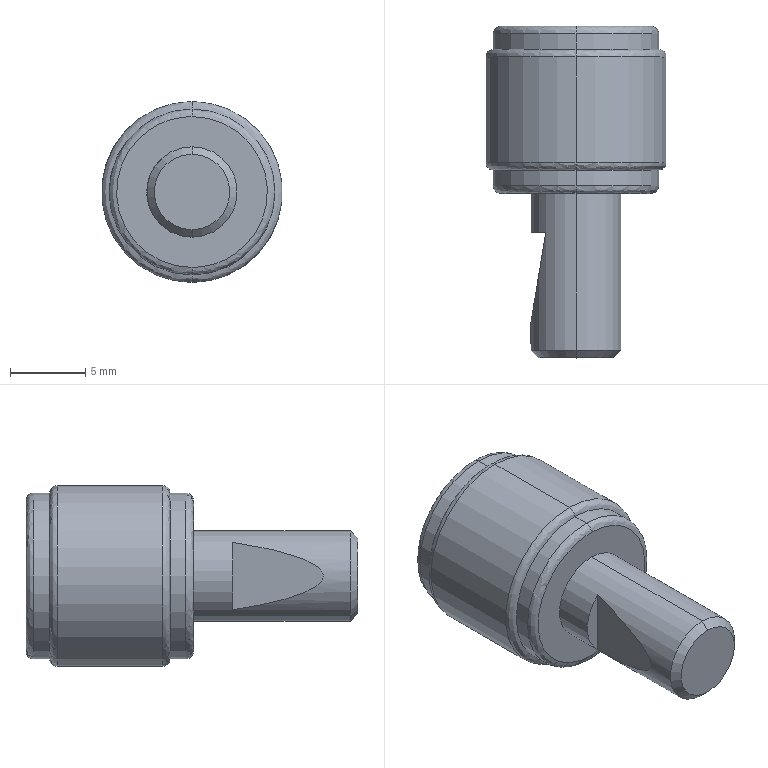Part | SolidWorks | features BaseBody 1 | 1 solid | 30 faces | box 12 x 22 x 12 mm | volume 1467 mm3 | plane 12 | spline 8 | cylinder 8 | cone 2 | commonest cylinder face diameters 11 x4 6 x2 12 x2
STEP:
#1=CARTESIAN_POINT('',(0.,20.45,5.5));
#2=VERTEX_POINT('',#1);
#3=CARTESIAN_POINT('',(0.,20.45,-5.5));
#4=VERTEX_POINT('',#3);
#5=CARTESIAN_POINT('',(0.,20.45,0.));
#6=DIRECTION('',(0.,-1.,0.));
#7=DIRECTION('',(0.,0.,1.));
#8=AXIS2_PLACEMENT_3D('',#5,#6,#7);
#9=CIRCLE('',#8,5.5);
#10=EDGE_CURVE('',#2,#4,#9,.T.);
#11=ORIENTED_EDGE('',*,*,#10,.T.);
#12=CARTESIAN_POINT('',(0.,19.95,-6.));
#13=VERTEX_POINT('',#12);
#14=CARTESIAN_POINT('',(0.,19.95,-5.5));
#15=DIRECTION('',(-1.,0.,0.));
#16=DIRECTION('',(0.,0.,-1.));
#17=AXIS2_PLACEMENT_3D('',#14,#15,#16);
#18=CIRCLE('',#17,0.5);
#19=EDGE_CURVE('',#4,#13,#18,.T.);
#20=ORIENTED_EDGE('',*,*,#19,.T.);
#21=CARTESIAN_POINT('',(0.,19.95,6.));
#22=VERTEX_POINT('',#21);
#23=CARTESIAN_POINT('',(0.,19.95,0.));
#24=DIRECTION('',(0.,-1.,0.));
#25=DIRECTION('',(0.,0.,1.));
#26=AXIS2_PLACEMENT_3D('',#23,#24,#25);
#27=CIRCLE('',#26,6.);
#28=EDGE_CURVE('',#22,#13,#27,.T.);
#29=ORIENTED_EDGE('',*,*,#28,.F.);
#30=CARTESIAN_POINT('',(0.,19.95,5.5));
#31=DIRECTION('',(1.,0.,0.));
#32=DIRECTION('',(0.,0.,1.));
#33=AXIS2_PLACEMENT_3D('',#30,#31,#32);
#34=CIRCLE('',#33,0.5);
#35=EDGE_CURVE('',#2,#22,#34,.T.);
#36=ORIENTED_EDGE('',*,*,#35,.F.);
#37=EDGE_LOOP('',(#11,#20,#29,#36));
#38=FACE_OUTER_BOUND('',#37,.T.);
#39=CARTESIAN_POINT('',(0.,20.45,-5.5));
#40=CARTESIAN_POINT('',(-11.,20.45,-5.5));
#41=CARTESIAN_POINT('',(-11.,20.45,5.5));
#42=CARTESIAN_POINT('',(0.,20.45,5.5));
#43=CARTESIAN_POINT('',(0.,20.45,-5.793));
#44=CARTESIAN_POINT('',(-11.586,20.45,-5.793));
#45=CARTESIAN_POINT('',(-11.586,20.45,5.793));
#46=CARTESIAN_POINT('',(0.,20.45,5.793));
#47=CARTESIAN_POINT('',(0.,20.243,-6.));
#48=CARTESIAN_POINT('',(-12.,20.243,-6.));
#49=CARTESIAN_POINT('',(-12.,20.243,6.));
#50=CARTESIAN_POINT('',(0.,20.243,6.));
#51=CARTESIAN_POINT('',(0.,19.95,-6.));
#52=CARTESIAN_POINT('',(-12.,19.95,-6.));
#53=CARTESIAN_POINT('',(-12.,19.95,6.));
#54=CARTESIAN_POINT('',(0.,19.95,6.));
#55=(BOUNDED_SURFACE()B_SPLINE_SURFACE(3,3,((#39,#40,#41,#42),(#43,#44,#45,#46),(#47,#48,#49,#50),(#51,#52,#53,#54)),.UNSPECIFIED.,.F.,.F.,.F.)B_SPLINE_SURFACE_WITH_KNOTS((4,4),(4,4),(0.,1.),(0.,1.),.UNSPECIFIED.)GEOMETRIC_REPRESENTATION_ITEM()RATIONAL_B_SPLINE_SURFACE(((1.,0.3333,0.3333,1.),(0.8047,0.2682,0.2682,0.8047),(0.8047,0.2682,0.2682,0.8047),(1.,0.3333,0.3333,1.)))REPRESENTATION_ITEM('')SURFACE());
#56=ADVANCED_FACE('',(#38),#55,.T.);
#57=CARTESIAN_POINT('',(0.,12.45,-5.5));
#58=VERTEX_POINT('',#57);
#59=CARTESIAN_POINT('',(0.,12.45,5.5));
#60=VERTEX_POINT('',#59);
#61=CARTESIAN_POINT('',(0.,12.45,0.));
#62=DIRECTION('',(0.,1.,0.));
#63=DIRECTION('',(0.,0.,-1.));
#64=AXIS2_PLACEMENT_3D('',#61,#62,#63);
#65=CIRCLE('',#64,5.5);
#66=EDGE_CURVE('',#58,#60,#65,.T.);
#67=ORIENTED_EDGE('',*,*,#66,.T.);
#68=CARTESIAN_POINT('',(0.,12.95,6.));
#69=VERTEX_POINT('',#68);
#70=CARTESIAN_POINT('',(0.,12.95,5.5));
#71=DIRECTION('',(-1.,0.,0.));
#72=DIRECTION('',(0.,0.,1.));
#73=AXIS2_PLACEMENT_3D('',#70,#71,#72);
#74=CIRCLE('',#73,0.5);
#75=EDGE_CURVE('',#60,#69,#74,.T.);
#76=ORIENTED_EDGE('',*,*,#75,.T.);
#77=CARTESIAN_POINT('',(0.,12.95,-6.));
#78=VERTEX_POINT('',#77);
#79=CARTESIAN_POINT('',(0.,12.95,0.));
#80=DIRECTION('',(0.,1.,0.));
#81=DIRECTION('',(0.,0.,1.));
#82=AXIS2_PLACEMENT_3D('',#79,#80,#81);
#83=CIRCLE('',#82,6.);
#84=EDGE_CURVE('',#78,#69,#83,.T.);
#85=ORIENTED_EDGE('',*,*,#84,.F.);
#86=CARTESIAN_POINT('',(0.,12.95,-5.5));
#87=DIRECTION('',(1.,0.,0.));
#88=DIRECTION('',(0.,0.,-1.));
#89=AXIS2_PLACEMENT_3D('',#86,#87,#88);
#90=CIRCLE('',#89,0.5);
#91=EDGE_CURVE('',#58,#78,#90,.T.);
#92=ORIENTED_EDGE('',*,*,#91,.F.);
#93=EDGE_LOOP('',(#67,#76,#85,#92));
#94=FACE_OUTER_BOUND('',#93,.T.);
#95=CARTESIAN_POINT('',(0.,12.45,5.5));
#96=CARTESIAN_POINT('',(-11.,12.45,5.5));
#97=CARTESIAN_POINT('',(-11.,12.45,-5.5));
#98=CARTESIAN_POINT('',(0.,12.45,-5.5));
#99=CARTESIAN_POINT('',(0.,12.45,5.793));
#100=CARTESIAN_POINT('',(-11.586,12.45,5.793));
#101=CARTESIAN_POINT('',(-11.586,12.45,-5.793));
#102=CARTESIAN_POINT('',(0.,12.45,-5.793));
#103=CARTESIAN_POINT('',(0.,12.657,6.));
#104=CARTESIAN_POINT('',(-12.,12.657,6.));
#105=CARTESIAN_POINT('',(-12.,12.657,-6.));
#106=CARTESIAN_POINT('',(0.,12.657,-6.));
#107=CARTESIAN_POINT('',(0.,12.95,6.));
#108=CARTESIAN_POINT('',(-12.,12.95,6.));
#109=CARTESIAN_POINT('',(-12.,12.95,-6.));
#110=CARTESIAN_POINT('',(0.,12.95,-6.));
#111=(BOUNDED_SURFACE()B_SPLINE_SURFACE(3,3,((#95,#96,#97,#98),(#99,#100,#101,#102),(#103,#104,#105,#106),(#107,#108,#109,#110)),.UNSPECIFIED.,.F.,.F.,.F.)B_SPLINE_SURFACE_WITH_KNOTS((4,4),(4,4),(0.,1.),(0.,1.),.UNSPECIFIED.)GEOMETRIC_REPRESENTATION_ITEM()RATIONAL_B_SPLINE_SURFACE(((1.,0.3333,0.3333,1.),(0.8047,0.2682,0.2682,0.8047),(0.8047,0.2682,0.2682,0.8047),(1.,0.3333,0.3333,1.)))REPRESENTATION_ITEM('')SURFACE());
#112=ADVANCED_FACE('',(#94),#111,.T.);
#113=CARTESIAN_POINT('',(0.,22.,5.));
#114=VERTEX_POINT('',#113);
#115=CARTESIAN_POINT('',(0.,22.,-5.));
#116=VERTEX_POINT('',#115);
#117=CARTESIAN_POINT('',(0.,22.,5.));
#118=CARTESIAN_POINT('',(-10.,22.,5.));
#119=CARTESIAN_POINT('',(-10.,22.,-5.));
#120=CARTESIAN_POINT('',(0.,22.,-5.));
#121=(BOUNDED_CURVE()B_SPLINE_CURVE(3,(#117,#118,#119,#120),.UNSPECIFIED.,.F.,.F.)B_SPLINE_CURVE_WITH_KNOTS((4,4),(0.,1.),.UNSPECIFIED.)CURVE()GEOMETRIC_REPRESENTATION_ITEM()RATIONAL_B_SPLINE_CURVE((1.,0.3333,0.3333,1.))REPRESENTATION_ITEM(''));
#122=EDGE_CURVE('',#114,#116,#121,.T.);
#123=ORIENTED_EDGE('',*,*,#122,.T.);
#124=CARTESIAN_POINT('',(0.,21.5,-5.5));
#125=VERTEX_POINT('',#124);
#126=CARTESIAN_POINT('',(0.,21.5,-5.));
#127=DIRECTION('',(-1.,0.,0.));
#128=DIRECTION('',(0.,0.,-1.));
#129=AXIS2_PLACEMENT_3D('',#126,#127,#128);
#130=CIRCLE('',#129,0.5);
#131=EDGE_CURVE('',#116,#125,#130,.T.);
#132=ORIENTED_EDGE('',*,*,#131,.T.);
#133=CARTESIAN_POINT('',(0.,21.5,5.5));
#134=VERTEX_POINT('',#133);
#135=CARTESIAN_POINT('',(0.,21.5,0.));
#136=DIRECTION('',(0.,-1.,0.));
#137=DIRECTION('',(0.,0.,1.));
#138=AXIS2_PLACEMENT_3D('',#135,#136,#137);
#139=CIRCLE('',#138,5.5);
#140=EDGE_CURVE('',#134,#125,#139,.T.);
#141=ORIENTED_EDGE('',*,*,#140,.F.);
#142=CARTESIAN_POINT('',(0.,21.5,5.));
#143=DIRECTION('',(1.,0.,0.));
#144=DIRECTION('',(0.,0.,1.));
#145=AXIS2_PLACEMENT_3D('',#142,#143,#144);
#146=CIRCLE('',#145,0.5);
#147=EDGE_CURVE('',#114,#134,#146,.T.);
#148=ORIENTED_EDGE('',*,*,#147,.F.);
#149=EDGE_LOOP('',(#123,#132,#141,#148));
#150=FACE_OUTER_BOUND('',#149,.T.);
#151=CARTESIAN_POINT('',(0.,22.,-5.));
#152=CARTESIAN_POINT('',(-10.,22.,-5.));
#153=CARTESIAN_POINT('',(-10.,22.,5.));
#154=CARTESIAN_POINT('',(0.,22.,5.));
#155=CARTESIAN_POINT('',(0.,22.,-5.293));
#156=CARTESIAN_POINT('',(-10.586,22.,-5.293));
#157=CARTESIAN_POINT('',(-10.586,22.,5.293));
#158=CARTESIAN_POINT('',(0.,22.,5.293));
#159=CARTESIAN_POINT('',(0.,21.793,-5.5));
#160=CARTESIAN_POINT('',(-11.,21.793,-5.5));
#161=CARTESIAN_POINT('',(-11.,21.793,5.5));
#162=CARTESIAN_POINT('',(0.,21.793,5.5));
#163=CARTESIAN_POINT('',(0.,21.5,-5.5));
#164=CARTESIAN_POINT('',(-11.,21.5,-5.5));
#165=CARTESIAN_POINT('',(-11.,21.5,5.5));
#166=CARTESIAN_POINT('',(0.,21.5,5.5));
#167=(BOUNDED_SURFACE()B_SPLINE_SURFACE(3,3,((#151,#152,#153,#154),(#155,#156,#157,#158),(#159,#160,#161,#162),(#163,#164,#165,#166)),.UNSPECIFIED.,.F.,.F.,.F.)B_SPLINE_SURFACE_WITH_KNOTS((4,4),(4,4),(0.,1.),(0.,1.),.UNSPECIFIED.)GEOMETRIC_REPRESENTATION_ITEM()RATIONAL_B_SPLINE_SURFACE(((1.,0.3333,0.3333,1.),(0.8047,0.2682,0.2682,0.8047),(0.8047,0.2682,0.2682,0.8047),(1.,0.3333,0.3333,1.)))REPRESENTATION_ITEM('')SURFACE());
#168=ADVANCED_FACE('',(#150),#167,.T.);
#169=CARTESIAN_POINT('',(0.,10.9,-5.));
#170=VERTEX_POINT('',#169);
#171=CARTESIAN_POINT('',(0.,10.9,5.));
#172=VERTEX_POINT('',#171);
#173=CARTESIAN_POINT('',(0.,10.9,-5.));
#174=CARTESIAN_POINT('',(-10.,10.9,-5.));
#175=CARTESIAN_POINT('',(-10.,10.9,5.));
#176=CARTESIAN_POINT('',(0.,10.9,5.));
#177=(BOUNDED_CURVE()B_SPLINE_CURVE(3,(#173,#174,#175,#176),.UNSPECIFIED.,.F.,.F.)B_SPLINE_CURVE_WITH_KNOTS((4,4),(0.,1.),.UNSPECIFIED.)CURVE()GEOMETRIC_REPRESENTATION_ITEM()RATIONAL_B_SPLINE_CURVE((1.,0.3333,0.3333,1.))REPRESENTATION_ITEM(''));
#178=EDGE_CURVE('',#170,#172,#177,.T.);
#179=ORIENTED_EDGE('',*,*,#178,.T.);
#180=CARTESIAN_POINT('',(0.,11.4,5.5));
#181=VERTEX_POINT('',#180);
#182=CARTESIAN_POINT('',(0.,11.4,5.));
#183=DIRECTION('',(-1.,0.,0.));
#184=DIRECTION('',(0.,0.,1.));
#185=AXIS2_PLACEMENT_3D('',#182,#183,#184);
#186=CIRCLE('',#185,0.5);
#187=EDGE_CURVE('',#172,#181,#186,.T.);
#188=ORIENTED_EDGE('',*,*,#187,.T.);
#189=CARTESIAN_POINT('',(0.,11.4,-5.5));
#190=VERTEX_POINT('',#189);
#191=CARTESIAN_POINT('',(0.,11.4,0.));
#192=DIRECTION('',(0.,1.,0.));
#193=DIRECTION('',(0.,0.,1.));
#194=AXIS2_PLACEMENT_3D('',#191,#192,#193);
#195=CIRCLE('',#194,5.5);
#196=EDGE_CURVE('',#190,#181,#195,.T.);
#197=ORIENTED_EDGE('',*,*,#196,.F.);
#198=CARTESIAN_POINT('',(0.,11.4,-5.));
#199=DIRECTION('',(1.,0.,0.));
#200=DIRECTION('',(0.,0.,-1.));
#201=AXIS2_PLACEMENT_3D('',#198,#199,#200);
#202=CIRCLE('',#201,0.5);
#203=EDGE_CURVE('',#170,#190,#202,.T.);
#204=ORIENTED_EDGE('',*,*,#203,.F.);
#205=EDGE_LOOP('',(#179,#188,#197,#204));
#206=FACE_OUTER_BOUND('',#205,.T.);
#207=CARTESIAN_POINT('',(0.,10.9,5.));
#208=CARTESIAN_POINT('',(-10.,10.9,5.));
#209=CARTESIAN_POINT('',(-10.,10.9,-5.));
#210=CARTESIAN_POINT('',(0.,10.9,-5.));
#211=CARTESIAN_POINT('',(0.,10.9,5.293));
#212=CARTESIAN_POINT('',(-10.586,10.9,5.293));
#213=CARTESIAN_POINT('',(-10.586,10.9,-5.293));
#214=CARTESIAN_POINT('',(0.,10.9,-5.293));
#215=CARTESIAN_POINT('',(0.,11.107,5.5));
#216=CARTESIAN_POINT('',(-11.,11.107,5.5));
#217=CARTESIAN_POINT('',(-11.,11.107,-5.5));
#218=CARTESIAN_POINT('',(0.,11.107,-5.5));
#219=CARTESIAN_POINT('',(0.,11.4,5.5));
#220=CARTESIAN_POINT('',(-11.,11.4,5.5));
#221=CARTESIAN_POINT('',(-11.,11.4,-5.5));
#222=CARTESIAN_POINT('',(0.,11.4,-5.5));
#223=(BOUNDED_SURFACE()B_SPLINE_SURFACE(3,3,((#207,#208,#209,#210),(#211,#212,#213,#214),(#215,#216,#217,#218),(#219,#220,#221,#222)),.UNSPECIFIED.,.F.,.F.,.F.)B_SPLINE_SURFACE_WITH_KNOTS((4,4),(4,4),(0.,1.),(0.,1.),.UNSPECIFIED.)GEOMETRIC_REPRESENTATION_ITEM()RATIONAL_B_SPLINE_SURFACE(((1.,0.3333,0.3333,1.),(0.8047,0.2682,0.2682,0.8047),(0.8047,0.2682,0.2682,0.8047),(1.,0.3333,0.3333,1.)))REPRESENTATION_ITEM('')SURFACE());
#224=ADVANCED_FACE('',(#206),#223,.T.);
#225=CARTESIAN_POINT('',(0.,12.95,0.));
#226=DIRECTION('',(0.,1.,0.));
#227=DIRECTION('',(0.,0.,1.));
#228=AXIS2_PLACEMENT_3D('',#225,#226,#227);
#229=CIRCLE('',#228,6.);
#230=EDGE_CURVE('',#69,#78,#229,.T.);
#231=ORIENTED_EDGE('',*,*,#230,.T.);
#232=CARTESIAN_POINT('',(0.,0.,-6.));
#233=DIRECTION('',(0.,1.,0.));
#234=VECTOR('',#233,1000.);
#235=LINE('',#232,#234);
#236=EDGE_CURVE('',#78,#13,#235,.T.);
#237=ORIENTED_EDGE('',*,*,#236,.T.);
#238=CARTESIAN_POINT('',(0.,19.95,0.));
#239=DIRECTION('',(0.,-1.,0.));
#240=DIRECTION('',(0.,0.,1.));
#241=AXIS2_PLACEMENT_3D('',#238,#239,#240);
#242=CIRCLE('',#241,6.);
#243=EDGE_CURVE('',#13,#22,#242,.T.);
#244=ORIENTED_EDGE('',*,*,#243,.T.);
#245=CARTESIAN_POINT('',(0.,0.,6.));
#246=DIRECTION('',(0.,1.,0.));
#247=VECTOR('',#246,1000.);
#248=LINE('',#245,#247);
#249=EDGE_CURVE('',#69,#22,#248,.T.);
#250=ORIENTED_EDGE('',*,*,#249,.F.);
#251=EDGE_LOOP('',(#231,#237,#244,#250));
#252=FACE_OUTER_BOUND('',#251,.T.);
#253=CARTESIAN_POINT('',(0.,0.,0.));
#254=DIRECTION('',(0.,1.,0.));
#255=DIRECTION('',(0.,0.,1.));
#256=AXIS2_PLACEMENT_3D('',#253,#254,#255);
#257=CYLINDRICAL_SURFACE('',#256,6.);
#258=ADVANCED_FACE('',(#252),#257,.T.);
#259=CARTESIAN_POINT('',(0.,20.45,0.));
#260=DIRECTION('',(0.,-1.,0.));
#261=DIRECTION('',(0.,0.,1.));
#262=AXIS2_PLACEMENT_3D('',#259,#260,#261);
#263=CIRCLE('',#262,5.5);
#264=EDGE_CURVE('',#4,#2,#263,.T.);
#265=ORIENTED_EDGE('',*,*,#264,.F.);
#266=CARTESIAN_POINT('',(0.,0.,-5.5));
#267=DIRECTION('',(0.,1.,0.));
#268=VECTOR('',#267,1000.);
#269=LINE('',#266,#268);
#270=EDGE_CURVE('',#4,#125,#269,.T.);
#271=ORIENTED_EDGE('',*,*,#270,.T.);
#272=CARTESIAN_POINT('',(0.,21.5,0.));
#273=DIRECTION('',(0.,-1.,0.));
#274=DIRECTION('',(0.,0.,1.));
#275=AXIS2_PLACEMENT_3D('',#272,#273,#274);
#276=CIRCLE('',#275,5.5);
#277=EDGE_CURVE('',#125,#134,#276,.T.);
#278=ORIENTED_EDGE('',*,*,#277,.T.);
#279=CARTESIAN_POINT('',(0.,0.,5.5));
#280=DIRECTION('',(0.,1.,0.));
#281=VECTOR('',#280,1000.);
#282=LINE('',#279,#281);
#283=EDGE_CURVE('',#2,#134,#282,.T.);
#284=ORIENTED_EDGE('',*,*,#283,.F.);
#285=EDGE_LOOP('',(#265,#271,#278,#284));
#286=FACE_OUTER_BOUND('',#285,.T.);
#287=CARTESIAN_POINT('',(0.,0.,0.));
#288=DIRECTION('',(0.,1.,0.));
#289=DIRECTION('',(0.,0.,1.));
#290=AXIS2_PLACEMENT_3D('',#287,#288,#289);
#291=CYLINDRICAL_SURFACE('',#290,5.5);
#292=ADVANCED_FACE('',(#286),#291,.T.);
#293=CARTESIAN_POINT('',(0.,11.4,0.));
#294=DIRECTION('',(0.,1.,0.));
#295=DIRECTION('',(0.,0.,1.));
#296=AXIS2_PLACEMENT_3D('',#293,#294,#295);
#297=CIRCLE('',#296,5.5);
#298=EDGE_CURVE('',#181,#190,#297,.T.);
#299=ORIENTED_EDGE('',*,*,#298,.T.);
#300=CARTESIAN_POINT('',(0.,0.,-5.5));
#301=DIRECTION('',(0.,1.,0.));
#302=VECTOR('',#301,1000.);
#303=LINE('',#300,#302);
#304=EDGE_CURVE('',#190,#58,#303,.T.);
#305=ORIENTED_EDGE('',*,*,#304,.T.);
#306=CARTESIAN_POINT('',(0.,12.45,0.));
#307=DIRECTION('',(0.,1.,0.));
#308=DIRECTION('',(0.,0.,-1.));
#309=AXIS2_PLACEMENT_3D('',#306,#307,#308);
#310=CIRCLE('',#309,5.5);
#311=EDGE_CURVE('',#60,#58,#310,.T.);
#312=ORIENTED_EDGE('',*,*,#311,.F.);
#313=CARTESIAN_POINT('',(0.,0.,5.5));
#314=DIRECTION('',(0.,1.,0.));
#315=VECTOR('',#314,1000.);
#316=LINE('',#313,#315);
#317=EDGE_CURVE('',#181,#60,#316,.T.);
#318=ORIENTED_EDGE('',*,*,#317,.F.);
#319=EDGE_LOOP('',(#299,#305,#312,#318));
#320=FACE_OUTER_BOUND('',#319,.T.);
#321=CARTESIAN_POINT('',(0.,0.,0.));
#322=DIRECTION('',(0.,1.,0.));
#323=DIRECTION('',(0.,0.,1.));
#324=AXIS2_PLACEMENT_3D('',#321,#322,#323);
#325=CYLINDRICAL_SURFACE('',#324,5.5);
#326=ADVANCED_FACE('',(#320),#325,.T.);
#327=CARTESIAN_POINT('',(0.,0.5,3.));
#328=VERTEX_POINT('',#327);
#329=CARTESIAN_POINT('',(0.,0.5,-3.));
#330=VERTEX_POINT('',#329);
#331=CARTESIAN_POINT('',(0.,0.5,0.));
#332=DIRECTION('',(0.,1.,0.));
#333=DIRECTION('',(0.,0.,1.));
#334=AXIS2_PLACEMENT_3D('',#331,#332,#333);
#335=CIRCLE('',#334,3.);
#336=EDGE_CURVE('',#328,#330,#335,.T.);
#337=ORIENTED_EDGE('',*,*,#336,.T.);
#338=CARTESIAN_POINT('',(0.,10.9,-3.));
#339=VERTEX_POINT('',#338);
#340=CARTESIAN_POINT('',(0.,0.,-3.));
#341=DIRECTION('',(0.,1.,0.));
#342=VECTOR('',#341,1000.);
#343=LINE('',#340,#342);
#344=EDGE_CURVE('',#330,#339,#343,.T.);
#345=ORIENTED_EDGE('',*,*,#344,.T.);
#346=CARTESIAN_POINT('',(0.,10.9,3.));
#347=VERTEX_POINT('',#346);
#348=CARTESIAN_POINT('',(0.,10.9,0.));
#349=DIRECTION('',(0.,1.,0.));
#350=DIRECTION('',(0.,0.,1.));
#351=AXIS2_PLACEMENT_3D('',#348,#349,#350);
#352=CIRCLE('',#351,3.);
#353=EDGE_CURVE('',#347,#339,#352,.T.);
#354=ORIENTED_EDGE('',*,*,#353,.F.);
#355=CARTESIAN_POINT('',(0.,0.,3.));
#356=DIRECTION('',(0.,1.,0.));
#357=VECTOR('',#356,1000.);
#358=LINE('',#355,#357);
#359=EDGE_CURVE('',#328,#347,#358,.T.);
#360=ORIENTED_EDGE('',*,*,#359,.F.);
#361=EDGE_LOOP('',(#337,#345,#354,#360));
#362=FACE_OUTER_BOUND('',#361,.T.);
#363=CARTESIAN_POINT('',(0.,0.,0.));
#364=DIRECTION('',(0.,1.,0.));
#365=DIRECTION('',(0.,0.,1.));
#366=AXIS2_PLACEMENT_3D('',#363,#364,#365);
#367=CYLINDRICAL_SURFACE('',#366,3.);
#368=ADVANCED_FACE('',(#362),#367,.T.);
#369=CARTESIAN_POINT('',(0.,0.,2.5));
#370=VERTEX_POINT('',#369);
#371=CARTESIAN_POINT('',(0.,0.,-2.5));
#372=VERTEX_POINT('',#371);
#373=CARTESIAN_POINT('',(0.,0.,0.));
#374=DIRECTION('',(0.,1.,0.));
#375=DIRECTION('',(0.,0.,1.));
#376=AXIS2_PLACEMENT_3D('',#373,#374,#375);
#377=CIRCLE('',#376,2.5);
#378=EDGE_CURVE('',#370,#372,#377,.T.);
#379=ORIENTED_EDGE('',*,*,#378,.T.);
#380=CARTESIAN_POINT('',(0.,0.5,-3.));
#381=DIRECTION('',(0.,0.7071,-0.7071));
#382=VECTOR('',#381,1000.);
#383=LINE('',#380,#382);
#384=EDGE_CURVE('',#372,#330,#383,.T.);
#385=ORIENTED_EDGE('',*,*,#384,.T.);
#386=ORIENTED_EDGE('',*,*,#336,.F.);
#387=CARTESIAN_POINT('',(0.,0.5,3.));
#388=DIRECTION('',(0.,0.7071,0.7071));
#389=VECTOR('',#388,1000.);
#390=LINE('',#387,#389);
#391=EDGE_CURVE('',#370,#328,#390,.T.);
#392=ORIENTED_EDGE('',*,*,#391,.F.);
#393=EDGE_LOOP('',(#379,#385,#386,#392));
#394=FACE_OUTER_BOUND('',#393,.T.);
#395=CARTESIAN_POINT('',(0.,0.5,0.));
#396=DIRECTION('',(0.,1.,0.));
#397=DIRECTION('',(0.,0.,1.));
#398=AXIS2_PLACEMENT_3D('',#395,#396,#397);
#399=CONICAL_SURFACE('',#398,3.,0.7854);
#400=ADVANCED_FACE('',(#394),#399,.T.);
#401=ORIENTED_EDGE('',*,*,#236,.F.);
#402=ORIENTED_EDGE('',*,*,#84,.T.);
#403=ORIENTED_EDGE('',*,*,#249,.T.);
#404=ORIENTED_EDGE('',*,*,#28,.T.);
#405=EDGE_LOOP('',(#401,#402,#403,#404));
#406=FACE_OUTER_BOUND('',#405,.T.);
#407=CARTESIAN_POINT('',(0.,0.,0.));
#408=DIRECTION('',(0.,1.,0.));
#409=DIRECTION('',(0.,0.,1.));
#410=AXIS2_PLACEMENT_3D('',#407,#408,#409);
#411=CYLINDRICAL_SURFACE('',#410,6.);
#412=ADVANCED_FACE('',(#406),#411,.T.);
#413=ORIENTED_EDGE('',*,*,#19,.F.);
#414=ORIENTED_EDGE('',*,*,#264,.T.);
#415=ORIENTED_EDGE('',*,*,#35,.T.);
#416=ORIENTED_EDGE('',*,*,#243,.F.);
#417=EDGE_LOOP('',(#413,#414,#415,#416));
#418=FACE_OUTER_BOUND('',#417,.T.);
#419=CARTESIAN_POINT('',(0.,20.45,5.5));
#420=CARTESIAN_POINT('',(11.,20.45,5.5));
#421=CARTESIAN_POINT('',(11.,20.45,-5.5));
#422=CARTESIAN_POINT('',(0.,20.45,-5.5));
#423=CARTESIAN_POINT('',(0.,20.45,5.793));
#424=CARTESIAN_POINT('',(11.586,20.45,5.793));
#425=CARTESIAN_POINT('',(11.586,20.45,-5.793));
#426=CARTESIAN_POINT('',(0.,20.45,-5.793));
#427=CARTESIAN_POINT('',(0.,20.243,6.));
#428=CARTESIAN_POINT('',(12.,20.243,6.));
#429=CARTESIAN_POINT('',(12.,20.243,-6.));
#430=CARTESIAN_POINT('',(0.,20.243,-6.));
#431=CARTESIAN_POINT('',(0.,19.95,6.));
#432=CARTESIAN_POINT('',(12.,19.95,6.));
#433=CARTESIAN_POINT('',(12.,19.95,-6.));
#434=CARTESIAN_POINT('',(0.,19.95,-6.));
#435=(BOUNDED_SURFACE()B_SPLINE_SURFACE(3,3,((#419,#420,#421,#422),(#423,#424,#425,#426),(#427,#428,#429,#430),(#431,#432,#433,#434)),.UNSPECIFIED.,.F.,.F.,.F.)B_SPLINE_SURFACE_WITH_KNOTS((4,4),(4,4),(0.,1.),(0.,1.),.UNSPECIFIED.)GEOMETRIC_REPRESENTATION_ITEM()RATIONAL_B_SPLINE_SURFACE(((1.,0.3333,0.3333,1.),(0.8047,0.2682,0.2682,0.8047),(0.8047,0.2682,0.2682,0.8047),(1.,0.3333,0.3333,1.)))REPRESENTATION_ITEM('')SURFACE());
#436=ADVANCED_FACE('',(#418),#435,.T.);
#437=ORIENTED_EDGE('',*,*,#75,.F.);
#438=ORIENTED_EDGE('',*,*,#311,.T.);
#439=ORIENTED_EDGE('',*,*,#91,.T.);
#440=ORIENTED_EDGE('',*,*,#230,.F.);
#441=EDGE_LOOP('',(#437,#438,#439,#440));
#442=FACE_OUTER_BOUND('',#441,.T.);
#443=CARTESIAN_POINT('',(0.,12.45,-5.5));
#444=CARTESIAN_POINT('',(11.,12.45,-5.5));
#445=CARTESIAN_POINT('',(11.,12.45,5.5));
#446=CARTESIAN_POINT('',(0.,12.45,5.5));
#447=CARTESIAN_POINT('',(0.,12.45,-5.793));
#448=CARTESIAN_POINT('',(11.586,12.45,-5.793));
#449=CARTESIAN_POINT('',(11.586,12.45,5.793));
#450=CARTESIAN_POINT('',(0.,12.45,5.793));
#451=CARTESIAN_POINT('',(0.,12.657,-6.));
#452=CARTESIAN_POINT('',(12.,12.657,-6.));
#453=CARTESIAN_POINT('',(12.,12.657,6.));
#454=CARTESIAN_POINT('',(0.,12.657,6.));
#455=CARTESIAN_POINT('',(0.,12.95,-6.));
#456=CARTESIAN_POINT('',(12.,12.95,-6.));
#457=CARTESIAN_POINT('',(12.,12.95,6.));
#458=CARTESIAN_POINT('',(0.,12.95,6.));
#459=(BOUNDED_SURFACE()B_SPLINE_SURFACE(3,3,((#443,#444,#445,#446),(#447,#448,#449,#450),(#451,#452,#453,#454),(#455,#456,#457,#458)),.UNSPECIFIED.,.F.,.F.,.F.)B_SPLINE_SURFACE_WITH_KNOTS((4,4),(4,4),(0.,1.),(0.,1.),.UNSPECIFIED.)GEOMETRIC_REPRESENTATION_ITEM()RATIONAL_B_SPLINE_SURFACE(((1.,0.3333,0.3333,1.),(0.8047,0.2682,0.2682,0.8047),(0.8047,0.2682,0.2682,0.8047),(1.,0.3333,0.3333,1.)))REPRESENTATION_ITEM('')SURFACE());
#460=ADVANCED_FACE('',(#442),#459,.T.);
#461=ORIENTED_EDGE('',*,*,#270,.F.);
#462=ORIENTED_EDGE('',*,*,#10,.F.);
#463=ORIENTED_EDGE('',*,*,#283,.T.);
#464=ORIENTED_EDGE('',*,*,#140,.T.);
#465=EDGE_LOOP('',(#461,#462,#463,#464));
#466=FACE_OUTER_BOUND('',#465,.T.);
#467=CARTESIAN_POINT('',(0.,0.,0.));
#468=DIRECTION('',(0.,1.,0.));
#469=DIRECTION('',(0.,0.,1.));
#470=AXIS2_PLACEMENT_3D('',#467,#468,#469);
#471=CYLINDRICAL_SURFACE('',#470,5.5);
#472=ADVANCED_FACE('',(#466),#471,.T.);
#473=ORIENTED_EDGE('',*,*,#304,.F.);
#474=ORIENTED_EDGE('',*,*,#196,.T.);
#475=ORIENTED_EDGE('',*,*,#317,.T.);
#476=ORIENTED_EDGE('',*,*,#66,.F.);
#477=EDGE_LOOP('',(#473,#474,#475,#476));
#478=FACE_OUTER_BOUND('',#477,.T.);
#479=CARTESIAN_POINT('',(0.,0.,0.));
#480=DIRECTION('',(0.,1.,0.));
#481=DIRECTION('',(0.,0.,1.));
#482=AXIS2_PLACEMENT_3D('',#479,#480,#481);
#483=CYLINDRICAL_SURFACE('',#482,5.5);
#484=ADVANCED_FACE('',(#478),#483,.T.);
#485=ORIENTED_EDGE('',*,*,#131,.F.);
#486=CARTESIAN_POINT('',(0.,22.,-5.));
#487=CARTESIAN_POINT('',(10.,22.,-5.));
#488=CARTESIAN_POINT('',(10.,22.,5.));
#489=CARTESIAN_POINT('',(0.,22.,5.));
#490=(BOUNDED_CURVE()B_SPLINE_CURVE(3,(#486,#487,#488,#489),.UNSPECIFIED.,.F.,.F.)B_SPLINE_CURVE_WITH_KNOTS((4,4),(0.,1.),.UNSPECIFIED.)CURVE()GEOMETRIC_REPRESENTATION_ITEM()RATIONAL_B_SPLINE_CURVE((1.,0.3333,0.3333,1.))REPRESENTATION_ITEM(''));
#491=EDGE_CURVE('',#116,#114,#490,.T.);
#492=ORIENTED_EDGE('',*,*,#491,.T.);
#493=ORIENTED_EDGE('',*,*,#147,.T.);
#494=ORIENTED_EDGE('',*,*,#277,.F.);
#495=EDGE_LOOP('',(#485,#492,#493,#494));
#496=FACE_OUTER_BOUND('',#495,.T.);
#497=CARTESIAN_POINT('',(0.,22.,5.));
#498=CARTESIAN_POINT('',(10.,22.,5.));
#499=CARTESIAN_POINT('',(10.,22.,-5.));
#500=CARTESIAN_POINT('',(0.,22.,-5.));
#501=CARTESIAN_POINT('',(0.,22.,5.293));
#502=CARTESIAN_POINT('',(10.586,22.,5.293));
#503=CARTESIAN_POINT('',(10.586,22.,-5.293));
#504=CARTESIAN_POINT('',(0.,22.,-5.293));
#505=CARTESIAN_POINT('',(0.,21.793,5.5));
#506=CARTESIAN_POINT('',(11.,21.793,5.5));
#507=CARTESIAN_POINT('',(11.,21.793,-5.5));
#508=CARTESIAN_POINT('',(0.,21.793,-5.5));
#509=CARTESIAN_POINT('',(0.,21.5,5.5));
#510=CARTESIAN_POINT('',(11.,21.5,5.5));
#511=CARTESIAN_POINT('',(11.,21.5,-5.5));
#512=CARTESIAN_POINT('',(0.,21.5,-5.5));
#513=(BOUNDED_SURFACE()B_SPLINE_SURFACE(3,3,((#497,#498,#499,#500),(#501,#502,#503,#504),(#505,#506,#507,#508),(#509,#510,#511,#512)),.UNSPECIFIED.,.F.,.F.,.F.)B_SPLINE_SURFACE_WITH_KNOTS((4,4),(4,4),(0.,1.),(0.,1.),.UNSPECIFIED.)GEOMETRIC_REPRESENTATION_ITEM()RATIONAL_B_SPLINE_SURFACE(((1.,0.3333,0.3333,1.),(0.8047,0.2682,0.2682,0.8047),(0.8047,0.2682,0.2682,0.8047),(1.,0.3333,0.3333,1.)))REPRESENTATION_ITEM('')SURFACE());
#514=ADVANCED_FACE('',(#496),#513,.T.);
#515=ORIENTED_EDGE('',*,*,#187,.F.);
#516=CARTESIAN_POINT('',(0.,10.9,5.));
#517=CARTESIAN_POINT('',(10.,10.9,5.));
#518=CARTESIAN_POINT('',(10.,10.9,-5.));
#519=CARTESIAN_POINT('',(0.,10.9,-5.));
#520=(BOUNDED_CURVE()B_SPLINE_CURVE(3,(#516,#517,#518,#519),.UNSPECIFIED.,.F.,.T.)B_SPLINE_CURVE_WITH_KNOTS((4,4),(0.,1.),.UNSPECIFIED.)CURVE()GEOMETRIC_REPRESENTATION_ITEM()RATIONAL_B_SPLINE_CURVE((1.,0.3333,0.3333,1.))REPRESENTATION_ITEM(''));
#521=EDGE_CURVE('',#172,#170,#520,.T.);
#522=ORIENTED_EDGE('',*,*,#521,.T.);
#523=ORIENTED_EDGE('',*,*,#203,.T.);
#524=ORIENTED_EDGE('',*,*,#298,.F.);
#525=EDGE_LOOP('',(#515,#522,#523,#524));
#526=FACE_OUTER_BOUND('',#525,.T.);
#527=CARTESIAN_POINT('',(0.,10.9,-5.));
#528=CARTESIAN_POINT('',(10.,10.9,-5.));
#529=CARTESIAN_POINT('',(10.,10.9,5.));
#530=CARTESIAN_POINT('',(0.,10.9,5.));
#531=CARTESIAN_POINT('',(0.,10.9,-5.293));
#532=CARTESIAN_POINT('',(10.586,10.9,-5.293));
#533=CARTESIAN_POINT('',(10.586,10.9,5.293));
#534=CARTESIAN_POINT('',(0.,10.9,5.293));
#535=CARTESIAN_POINT('',(0.,11.107,-5.5));
#536=CARTESIAN_POINT('',(11.,11.107,-5.5));
#537=CARTESIAN_POINT('',(11.,11.107,5.5));
#538=CARTESIAN_POINT('',(0.,11.107,5.5));
#539=CARTESIAN_POINT('',(0.,11.4,-5.5));
#540=CARTESIAN_POINT('',(11.,11.4,-5.5));
#541=CARTESIAN_POINT('',(11.,11.4,5.5));
#542=CARTESIAN_POINT('',(0.,11.4,5.5));
#543=(BOUNDED_SURFACE()B_SPLINE_SURFACE(3,3,((#527,#528,#529,#530),(#531,#532,#533,#534),(#535,#536,#537,#538),(#539,#540,#541,#542)),.UNSPECIFIED.,.F.,.F.,.F.)B_SPLINE_SURFACE_WITH_KNOTS((4,4),(4,4),(0.,1.),(0.,1.),.UNSPECIFIED.)GEOMETRIC_REPRESENTATION_ITEM()RATIONAL_B_SPLINE_SURFACE(((1.,0.3333,0.3333,1.),(0.8047,0.2682,0.2682,0.8047),(0.8047,0.2682,0.2682,0.8047),(1.,0.3333,0.3333,1.)))REPRESENTATION_ITEM('')SURFACE());
#544=ADVANCED_FACE('',(#526),#543,.T.);
#545=ORIENTED_EDGE('',*,*,#491,.F.);
#546=ORIENTED_EDGE('',*,*,#122,.F.);
#547=EDGE_LOOP('',(#545,#546));
#548=FACE_OUTER_BOUND('',#547,.T.);
#549=CARTESIAN_POINT('',(-0.866,22.,-1.5));
#550=VERTEX_POINT('',#549);
#551=CARTESIAN_POINT('',(0.866,22.,-1.5));
#552=VERTEX_POINT('',#551);
#553=CARTESIAN_POINT('',(0.866,22.,-1.5));
#554=DIRECTION('',(1.,0.,0.));
#555=VECTOR('',#554,1000.);
#556=LINE('',#553,#555);
#557=EDGE_CURVE('',#550,#552,#556,.T.);
#558=ORIENTED_EDGE('',*,*,#557,.T.);
#559=CARTESIAN_POINT('',(1.732,22.,0.));
#560=VERTEX_POINT('',#559);
#561=CARTESIAN_POINT('',(0.866,22.,-1.5));
#562=DIRECTION('',(0.5,0.,0.866));
#563=VECTOR('',#562,1000.);
#564=LINE('',#561,#563);
#565=EDGE_CURVE('',#552,#560,#564,.T.);
#566=ORIENTED_EDGE('',*,*,#565,.T.);
#567=CARTESIAN_POINT('',(0.866,22.,1.5));
#568=VERTEX_POINT('',#567);
#569=CARTESIAN_POINT('',(0.866,22.,1.5));
#570=DIRECTION('',(-0.5,0.,0.866));
#571=VECTOR('',#570,1000.);
#572=LINE('',#569,#571);
#573=EDGE_CURVE('',#560,#568,#572,.T.);
#574=ORIENTED_EDGE('',*,*,#573,.T.);
#575=CARTESIAN_POINT('',(-0.866,22.,1.5));
#576=VERTEX_POINT('',#575);
#577=CARTESIAN_POINT('',(-0.866,22.,1.5));
#578=DIRECTION('',(-1.,0.,0.));
#579=VECTOR('',#578,1000.);
#580=LINE('',#577,#579);
#581=EDGE_CURVE('',#568,#576,#580,.T.);
#582=ORIENTED_EDGE('',*,*,#581,.T.);
#583=CARTESIAN_POINT('',(-1.732,22.,0.));
#584=VERTEX_POINT('',#583);
#585=CARTESIAN_POINT('',(-1.732,22.,0.));
#586=DIRECTION('',(-0.5,0.,-0.866));
#587=VECTOR('',#586,1000.);
#588=LINE('',#585,#587);
#589=EDGE_CURVE('',#576,#584,#588,.T.);
#590=ORIENTED_EDGE('',*,*,#589,.T.);
#591=CARTESIAN_POINT('',(-0.866,22.,-1.5));
#592=DIRECTION('',(0.5,0.,-0.866));
#593=VECTOR('',#592,1000.);
#594=LINE('',#591,#593);
#595=EDGE_CURVE('',#584,#550,#594,.T.);
#596=ORIENTED_EDGE('',*,*,#595,.T.);
#597=EDGE_LOOP('',(#558,#566,#574,#582,#590,#596));
#598=FACE_BOUND('',#597,.T.);
#599=CARTESIAN_POINT('',(0.,22.,0.));
#600=DIRECTION('',(0.,1.,0.));
#601=DIRECTION('',(0.,0.,1.));
#602=AXIS2_PLACEMENT_3D('',#599,#600,#601);
#603=PLANE('',#602);
#604=ADVANCED_FACE('',(#548,#598),#603,.T.);
#605=ORIENTED_EDGE('',*,*,#353,.T.);
#606=CARTESIAN_POINT('',(0.,10.9,0.));
#607=DIRECTION('',(0.,1.,0.));
#608=DIRECTION('',(0.,0.,1.));
#609=AXIS2_PLACEMENT_3D('',#606,#607,#608);
#610=CIRCLE('',#609,3.);
#611=EDGE_CURVE('',#339,#347,#610,.T.);
#612=ORIENTED_EDGE('',*,*,#611,.T.);
#613=EDGE_LOOP('',(#605,#612));
#614=FACE_BOUND('',#613,.T.);
#615=ORIENTED_EDGE('',*,*,#521,.F.);
#616=ORIENTED_EDGE('',*,*,#178,.F.);
#617=EDGE_LOOP('',(#615,#616));
#618=FACE_OUTER_BOUND('',#617,.T.);
#619=CARTESIAN_POINT('',(-5.5,10.9,0.));
#620=DIRECTION('',(0.,-1.,0.));
#621=DIRECTION('',(0.,0.,-1.));
#622=AXIS2_PLACEMENT_3D('',#619,#620,#621);
#623=PLANE('',#622);
#624=ADVANCED_FACE('',(#614,#618),#623,.T.);
#625=CARTESIAN_POINT('',(0.866,19.,-1.5));
#626=VERTEX_POINT('',#625);
#627=CARTESIAN_POINT('',(0.866,19.,-1.5));
#628=DIRECTION('',(0.,1.,0.));
#629=VECTOR('',#628,1000.);
#630=LINE('',#627,#629);
#631=EDGE_CURVE('',#626,#552,#630,.T.);
#632=ORIENTED_EDGE('',*,*,#631,.F.);
#633=CARTESIAN_POINT('',(1.732,19.,0.));
#634=VERTEX_POINT('',#633);
#635=CARTESIAN_POINT('',(1.732,19.,0.));
#636=DIRECTION('',(-0.5,0.,-0.866));
#637=VECTOR('',#636,1000.);
#638=LINE('',#635,#637);
#639=EDGE_CURVE('',#634,#626,#638,.T.);
#640=ORIENTED_EDGE('',*,*,#639,.F.);
#641=CARTESIAN_POINT('',(1.732,19.,0.));
#642=DIRECTION('',(0.,-1.,0.));
#643=VECTOR('',#642,1000.);
#644=LINE('',#641,#643);
#645=EDGE_CURVE('',#560,#634,#644,.T.);
#646=ORIENTED_EDGE('',*,*,#645,.F.);
#647=ORIENTED_EDGE('',*,*,#565,.F.);
#648=EDGE_LOOP('',(#632,#640,#646,#647));
#649=FACE_OUTER_BOUND('',#648,.T.);
#650=CARTESIAN_POINT('',(1.732,19.,0.));
#651=DIRECTION('',(0.866,0.,-0.5));
#652=DIRECTION('',(-0.5,0.,-0.866));
#653=AXIS2_PLACEMENT_3D('',#650,#651,#652);
#654=PLANE('',#653);
#655=ADVANCED_FACE('',(#649),#654,.F.);
#656=ORIENTED_EDGE('',*,*,#344,.F.);
#657=CARTESIAN_POINT('',(0.,0.5,0.));
#658=DIRECTION('',(0.,1.,0.));
#659=DIRECTION('',(0.,0.,1.));
#660=AXIS2_PLACEMENT_3D('',#657,#658,#659);
#661=CIRCLE('',#660,3.);
#662=EDGE_CURVE('',#330,#328,#661,.T.);
#663=ORIENTED_EDGE('',*,*,#662,.T.);
#664=ORIENTED_EDGE('',*,*,#359,.T.);
#665=ORIENTED_EDGE('',*,*,#611,.F.);
#666=EDGE_LOOP('',(#656,#663,#664,#665));
#667=FACE_OUTER_BOUND('',#666,.T.);
#668=CARTESIAN_POINT('',(-2.,8.3,2.236));
#669=VERTEX_POINT('',#668);
#670=CARTESIAN_POINT('',(-2.,8.3,-2.236));
#671=VERTEX_POINT('',#670);
#672=CARTESIAN_POINT('',(-2.,8.3,2.236));
#673=CARTESIAN_POINT('',(-3.429,-0.2714,0.9583));
#674=CARTESIAN_POINT('',(-3.429,-0.2714,-0.9583));
#675=CARTESIAN_POINT('',(-2.,8.3,-2.236));
#676=(BOUNDED_CURVE()B_SPLINE_CURVE(3,(#672,#673,#674,#675),.UNSPECIFIED.,.F.,.F.)B_SPLINE_CURVE_WITH_KNOTS((4,4),(2.301,3.983),.UNSPECIFIED.)CURVE()GEOMETRIC_REPRESENTATION_ITEM()RATIONAL_B_SPLINE_CURVE((1.,0.7778,0.7778,1.))REPRESENTATION_ITEM(''));
#677=EDGE_CURVE('',#669,#671,#676,.T.);
#678=ORIENTED_EDGE('',*,*,#677,.T.);
#679=CARTESIAN_POINT('',(0.,8.3,0.));
#680=DIRECTION('',(0.,1.,0.));
#681=DIRECTION('',(0.,0.,1.));
#682=AXIS2_PLACEMENT_3D('',#679,#680,#681);
#683=CIRCLE('',#682,3.);
#684=EDGE_CURVE('',#671,#669,#683,.T.);
#685=ORIENTED_EDGE('',*,*,#684,.T.);
#686=EDGE_LOOP('',(#678,#685));
#687=FACE_BOUND('',#686,.T.);
#688=CARTESIAN_POINT('',(0.,0.,0.));
#689=DIRECTION('',(0.,1.,0.));
#690=DIRECTION('',(0.,0.,1.));
#691=AXIS2_PLACEMENT_3D('',#688,#689,#690);
#692=CYLINDRICAL_SURFACE('',#691,3.);
#693=ADVANCED_FACE('',(#667,#687),#692,.T.);
#694=CARTESIAN_POINT('',(-0.866,19.,-1.5));
#695=VERTEX_POINT('',#694);
#696=CARTESIAN_POINT('',(-0.866,19.,-1.5));
#697=DIRECTION('',(0.,1.,0.));
#698=VECTOR('',#697,1000.);
#699=LINE('',#696,#698);
#700=EDGE_CURVE('',#695,#550,#699,.T.);
#701=ORIENTED_EDGE('',*,*,#700,.F.);
#702=CARTESIAN_POINT('',(0.866,19.,-1.5));
#703=DIRECTION('',(-1.,0.,0.));
#704=VECTOR('',#703,1000.);
#705=LINE('',#702,#704);
#706=EDGE_CURVE('',#626,#695,#705,.T.);
#707=ORIENTED_EDGE('',*,*,#706,.F.);
#708=ORIENTED_EDGE('',*,*,#631,.T.);
#709=ORIENTED_EDGE('',*,*,#557,.F.);
#710=EDGE_LOOP('',(#701,#707,#708,#709));
#711=FACE_OUTER_BOUND('',#710,.T.);
#712=CARTESIAN_POINT('',(0.866,19.,-1.5));
#713=DIRECTION('',(0.,0.,-1.));
#714=DIRECTION('',(-1.,0.,0.));
#715=AXIS2_PLACEMENT_3D('',#712,#713,#714);
#716=PLANE('',#715);
#717=ADVANCED_FACE('',(#711),#716,.F.);
#718=CARTESIAN_POINT('',(-1.732,19.,0.));
#719=VERTEX_POINT('',#718);
#720=CARTESIAN_POINT('',(-0.866,19.,1.5));
#721=VERTEX_POINT('',#720);
#722=CARTESIAN_POINT('',(-1.732,19.,0.));
#723=DIRECTION('',(0.5,0.,0.866));
#724=VECTOR('',#723,1000.);
#725=LINE('',#722,#724);
#726=EDGE_CURVE('',#719,#721,#725,.T.);
#727=ORIENTED_EDGE('',*,*,#726,.T.);
#728=CARTESIAN_POINT('',(0.866,19.,1.5));
#729=VERTEX_POINT('',#728);
#730=CARTESIAN_POINT('',(-0.866,19.,1.5));
#731=DIRECTION('',(1.,0.,0.));
#732=VECTOR('',#731,1000.);
#733=LINE('',#730,#732);
#734=EDGE_CURVE('',#721,#729,#733,.T.);
#735=ORIENTED_EDGE('',*,*,#734,.T.);
#736=CARTESIAN_POINT('',(0.866,19.,1.5));
#737=DIRECTION('',(0.5,0.,-0.866));
#738=VECTOR('',#737,1000.);
#739=LINE('',#736,#738);
#740=EDGE_CURVE('',#729,#634,#739,.T.);
#741=ORIENTED_EDGE('',*,*,#740,.T.);
#742=ORIENTED_EDGE('',*,*,#639,.T.);
#743=ORIENTED_EDGE('',*,*,#706,.T.);
#744=CARTESIAN_POINT('',(-0.866,19.,-1.5));
#745=DIRECTION('',(-0.5,0.,0.866));
#746=VECTOR('',#745,1000.);
#747=LINE('',#744,#746);
#748=EDGE_CURVE('',#695,#719,#747,.T.);
#749=ORIENTED_EDGE('',*,*,#748,.T.);
#750=EDGE_LOOP('',(#727,#735,#741,#742,#743,#749));
#751=FACE_OUTER_BOUND('',#750,.T.);
#752=CARTESIAN_POINT('',(0.,19.,0.));
#753=DIRECTION('',(0.,1.,0.));
#754=DIRECTION('',(0.,0.,1.));
#755=AXIS2_PLACEMENT_3D('',#752,#753,#754);
#756=PLANE('',#755);
#757=ADVANCED_FACE('',(#751),#756,.T.);
#758=ORIENTED_EDGE('',*,*,#645,.T.);
#759=ORIENTED_EDGE('',*,*,#740,.F.);
#760=CARTESIAN_POINT('',(0.866,19.,1.5));
#761=DIRECTION('',(0.,-1.,0.));
#762=VECTOR('',#761,1000.);
#763=LINE('',#760,#762);
#764=EDGE_CURVE('',#568,#729,#763,.T.);
#765=ORIENTED_EDGE('',*,*,#764,.F.);
#766=ORIENTED_EDGE('',*,*,#573,.F.);
#767=EDGE_LOOP('',(#758,#759,#765,#766));
#768=FACE_OUTER_BOUND('',#767,.T.);
#769=CARTESIAN_POINT('',(0.866,19.,1.5));
#770=DIRECTION('',(0.866,0.,0.5));
#771=DIRECTION('',(0.5,0.,-0.866));
#772=AXIS2_PLACEMENT_3D('',#769,#770,#771);
#773=PLANE('',#772);
#774=ADVANCED_FACE('',(#768),#773,.F.);
#775=ORIENTED_EDGE('',*,*,#684,.F.);
#776=CARTESIAN_POINT('',(-2.,8.3,-6.));
#777=DIRECTION('',(0.,0.,-1.));
#778=VECTOR('',#777,1000.);
#779=LINE('',#776,#778);
#780=EDGE_CURVE('',#669,#671,#779,.T.);
#781=ORIENTED_EDGE('',*,*,#780,.F.);
#782=EDGE_LOOP('',(#775,#781));
#783=FACE_OUTER_BOUND('',#782,.T.);
#784=CARTESIAN_POINT('',(-3.,8.3,-6.));
#785=DIRECTION('',(0.,1.,0.));
#786=DIRECTION('',(0.,0.,1.));
#787=AXIS2_PLACEMENT_3D('',#784,#785,#786);
#788=PLANE('',#787);
#789=ADVANCED_FACE('',(#783),#788,.F.);
#790=ORIENTED_EDGE('',*,*,#677,.F.);
#791=ORIENTED_EDGE('',*,*,#780,.T.);
#792=EDGE_LOOP('',(#790,#791));
#793=FACE_OUTER_BOUND('',#792,.T.);
#794=CARTESIAN_POINT('',(-2.,8.3,-6.));
#795=DIRECTION('',(0.9864,-0.1644,0.));
#796=DIRECTION('',(0.1644,0.9864,0.));
#797=AXIS2_PLACEMENT_3D('',#794,#795,#796);
#798=PLANE('',#797);
#799=ADVANCED_FACE('',(#793),#798,.F.);
#800=ORIENTED_EDGE('',*,*,#384,.F.);
#801=CARTESIAN_POINT('',(0.,0.,0.));
#802=DIRECTION('',(0.,1.,0.));
#803=DIRECTION('',(0.,0.,1.));
#804=AXIS2_PLACEMENT_3D('',#801,#802,#803);
#805=CIRCLE('',#804,2.5);
#806=EDGE_CURVE('',#372,#370,#805,.T.);
#807=ORIENTED_EDGE('',*,*,#806,.T.);
#808=ORIENTED_EDGE('',*,*,#391,.T.);
#809=ORIENTED_EDGE('',*,*,#662,.F.);
#810=EDGE_LOOP('',(#800,#807,#808,#809));
#811=FACE_OUTER_BOUND('',#810,.T.);
#812=CARTESIAN_POINT('',(0.,0.5,0.));
#813=DIRECTION('',(0.,1.,0.));
#814=DIRECTION('',(0.,0.,1.));
#815=AXIS2_PLACEMENT_3D('',#812,#813,#814);
#816=CONICAL_SURFACE('',#815,3.,0.7854);
#817=ADVANCED_FACE('',(#811),#816,.T.);
#818=CARTESIAN_POINT('',(-1.732,19.,0.));
#819=DIRECTION('',(0.,1.,0.));
#820=VECTOR('',#819,1000.);
#821=LINE('',#818,#820);
#822=EDGE_CURVE('',#719,#584,#821,.T.);
#823=ORIENTED_EDGE('',*,*,#822,.F.);
#824=ORIENTED_EDGE('',*,*,#748,.F.);
#825=ORIENTED_EDGE('',*,*,#700,.T.);
#826=ORIENTED_EDGE('',*,*,#595,.F.);
#827=EDGE_LOOP('',(#823,#824,#825,#826));
#828=FACE_OUTER_BOUND('',#827,.T.);
#829=CARTESIAN_POINT('',(-0.866,19.,-1.5));
#830=DIRECTION('',(-0.866,0.,-0.5));
#831=DIRECTION('',(-0.5,0.,0.866));
#832=AXIS2_PLACEMENT_3D('',#829,#830,#831);
#833=PLANE('',#832);
#834=ADVANCED_FACE('',(#828),#833,.F.);
#835=ORIENTED_EDGE('',*,*,#764,.T.);
#836=ORIENTED_EDGE('',*,*,#734,.F.);
#837=CARTESIAN_POINT('',(-0.866,19.,1.5));
#838=DIRECTION('',(0.,-1.,0.));
#839=VECTOR('',#838,1000.);
#840=LINE('',#837,#839);
#841=EDGE_CURVE('',#576,#721,#840,.T.);
#842=ORIENTED_EDGE('',*,*,#841,.F.);
#843=ORIENTED_EDGE('',*,*,#581,.F.);
#844=EDGE_LOOP('',(#835,#836,#842,#843));
#845=FACE_OUTER_BOUND('',#844,.T.);
#846=CARTESIAN_POINT('',(-0.866,19.,1.5));
#847=DIRECTION('',(0.,0.,1.));
#848=DIRECTION('',(1.,0.,0.));
#849=AXIS2_PLACEMENT_3D('',#846,#847,#848);
#850=PLANE('',#849);
#851=ADVANCED_FACE('',(#845),#850,.F.);
#852=ORIENTED_EDGE('',*,*,#378,.F.);
#853=ORIENTED_EDGE('',*,*,#806,.F.);
#854=EDGE_LOOP('',(#852,#853));
#855=FACE_OUTER_BOUND('',#854,.T.);
#856=CARTESIAN_POINT('',(-3.,0.,0.));
#857=DIRECTION('',(0.,-1.,0.));
#858=DIRECTION('',(0.,0.,-1.));
#859=AXIS2_PLACEMENT_3D('',#856,#857,#858);
#860=PLANE('',#859);
#861=ADVANCED_FACE('',(#855),#860,.T.);
#862=ORIENTED_EDGE('',*,*,#841,.T.);
#863=ORIENTED_EDGE('',*,*,#726,.F.);
#864=ORIENTED_EDGE('',*,*,#822,.T.);
#865=ORIENTED_EDGE('',*,*,#589,.F.);
#866=EDGE_LOOP('',(#862,#863,#864,#865));
#867=FACE_OUTER_BOUND('',#866,.T.);
#868=CARTESIAN_POINT('',(-1.732,19.,0.));
#869=DIRECTION('',(-0.866,0.,0.5));
#870=DIRECTION('',(0.5,0.,0.866));
#871=AXIS2_PLACEMENT_3D('',#868,#869,#870);
#872=PLANE('',#871);
#873=ADVANCED_FACE('',(#867),#872,.F.);
#874=CLOSED_SHELL('',(#56,#112,#168,#224,#258,#292,#326,#368,#400,#412,#436,#460,#472,#484,#514,#544,#604,#624,#655,#693,#717,#757,#774,#789,#799,#817,#834,#851,#861,#873));
#875=MANIFOLD_SOLID_BREP('',#874);
#876=CARTESIAN_POINT('',(0.,0.,0.));
#877=DIRECTION('',(0.,0.,1.));
#878=DIRECTION('',(1.,0.,0.));
#879=AXIS2_PLACEMENT_3D('',#876,#877,#878);
#880=(LENGTH_UNIT()NAMED_UNIT(*)SI_UNIT(.MILLI.,.METRE.));
#881=UNCERTAINTY_MEASURE_WITH_UNIT(LENGTH_MEASURE(0.00001),#880,'','');
#882=(NAMED_UNIT(*)PLANE_ANGLE_UNIT()SI_UNIT($,.RADIAN.));
#883=(NAMED_UNIT(*)SI_UNIT($,.STERADIAN.)SOLID_ANGLE_UNIT());
#884=(GEOMETRIC_REPRESENTATION_CONTEXT(3)GLOBAL_UNCERTAINTY_ASSIGNED_CONTEXT((#881))GLOBAL_UNIT_ASSIGNED_CONTEXT((#880,#882,#883))REPRESENTATION_CONTEXT('',''));
#885=ADVANCED_BREP_SHAPE_REPRESENTATION('',(#875,#879),#884);